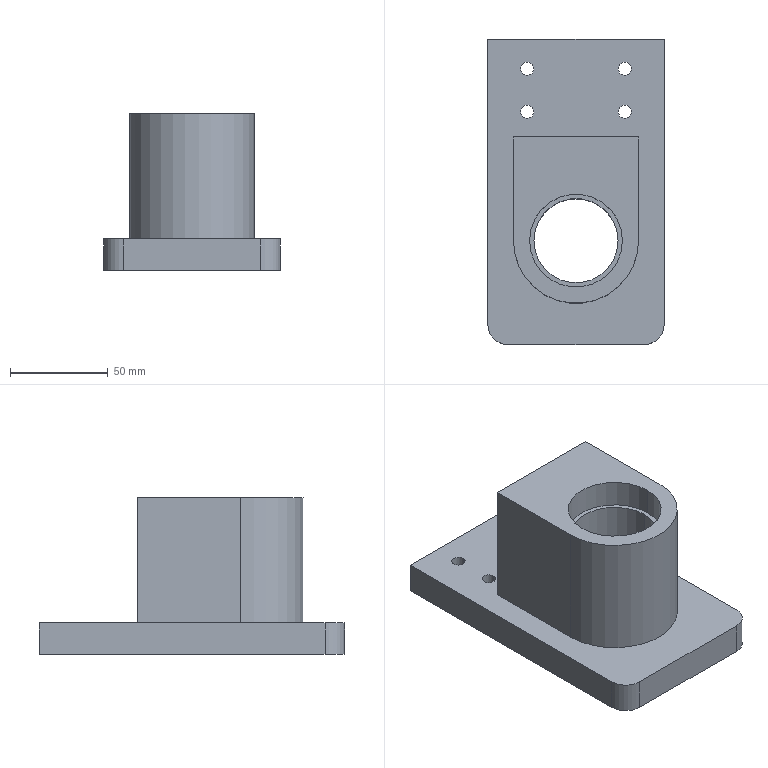NC program | NX | posted with a generic post | part box 90 x 156 x 80 mm
Lines 1 to 810 of 2108:
N10 G17 G21 G94 G90
(ADAPTIVE_MILLING , TOOL : D12-36-D12-120-3T-FINISH)
N12 T05 M6
N14 G54
N16 G17 G0 G90 X78.744 Y-62.046 S3000 M3
N18 G43 Z30. H5
N20 Z3.2
N22 G94 G1 X78.746 Y-61.896 Z2.263 F2000.
N24 X78.749 Y-61.746 Z1.892
N26 X78.751 Y-61.596 Z1.62
N28 X78.753 Y-61.446 Z1.4
N30 X78.756 Y-61.296 Z1.216
N32 X78.758 Y-61.146 Z1.058
N34 X78.76 Y-60.996 Z0.92
N36 X78.763 Y-60.846 Z0.8
N38 X78.765 Y-60.696 Z0.695
N40 X78.767 Y-60.546 Z0.602
N42 X78.77 Y-60.396 Z0.521
N44 X78.772 Y-60.246 Z0.45
N46 X78.774 Y-60.096 Z0.39
N48 X78.777 Y-59.946 Z0.338
N50 X78.779 Y-59.796 Z0.295
N52 X78.782 Y-59.646 Z0.261
N54 X78.784 Y-59.496 Z0.234
N56 X78.786 Y-59.346 Z0.215
N58 X78.789 Y-59.197 Z0.204
N60 X78.791 Y-59.047 Z0.2
N62 X78.82 Y-57.201
N64 G3 X77.983 Y-56.029 R1.212
N66 X74.762 Y-55.55 R13.285
N68 X65.236 Y-55.402 R193.444
N70 G1 X60.785 Y-55.4
N72 X-78.76 Y-55.399
N74 G2 X-83.906 Y-52.932 R6.712
N76 X-86.208 Y-48.01 R11.134
N78 X-86.816 Y-42.064 R32.789
N80 X-86.9 Y-29.285 R524.641
N82 G1 X-86.898 Y47.291
N84 G2 X-84.476 Y52.367 R6.698
N86 X-79.698 Y54.664 R10.957
N88 X-73.892 Y55.305 R30.703
N90 X-60.843 Y55.4 R460.922
N92 G1 X78.741 Y55.399
N94 G2 X83.892 Y52.944 R6.704
N96 X86.203 Y48.02 R11.142
N98 X86.818 Y41.985 R32.906
N100 X86.9 Y29.386 R528.978
N102 G1 X86.899 Y-47.241
N104 G2 X84.478 Y-52.363 R6.699
N106 X79.822 Y-54.481 R9.521
N108 X74.441 Y-54.838 R30.69
N110 G1 X63.303 Y-54.802
N112 X-76.33 Y-54.8
N114 G2 X-83.402 Y-51.047 R8.604
N116 X-85.614 Y-45.563 R13.915
N118 X-86.224 Y-38.713 R42.06
N120 X-86.299 Y-25.843 R645.049
N122 G1 X-86.298 Y44.918
N124 G2 X-82.556 Y51.894 R8.601
N126 X-77.072 Y54.112 R13.896
N128 X-70.357 Y54.72 R41.378
N130 X-57.488 Y54.799 R603.139
N132 G1 X76.413 Y54.798
N134 G2 X83.395 Y51.052 R8.603
N136 X85.602 Y45.614 R13.877
N138 X86.221 Y38.81 R41.342
N140 X86.299 Y26.166 R605.307
N142 G1 X86.298 Y-44.913
N144 G2 X82.262 Y-51.953 R8.28
N146 X76.935 Y-53.785 R13.806
N148 X70.203 Y-54.183 R49.593
N150 G1 X60.966 Y-54.2
N152 X-74.139 Y-54.199
N154 G2 X-83.054 Y-49.203 R9.955
N156 X-85.085 Y-43.278 R16.664
N158 X-85.637 Y-35.79 R53.798
N160 X-85.699 Y-22.92 R771.076
N162 G1 X-85.697 Y42.759
N164 G2 X-80.83 Y51.476 R9.919
N166 X-75.008 Y53.546 R16.303
N168 X-67.793 Y54.125 R49.758
N170 X-55.733 Y54.198 R669.374
N172 G1 X74.254 Y54.197
N174 G2 X83.001 Y49.286 R9.929
N176 X85.082 Y43.287 R16.583
N178 X85.634 Y35.889 R53.121
N180 X85.699 Y23.514 R746.255
N182 G1 X85.697 Y-42.753
N184 G2 X80.99 Y-51.128 R9.462
N186 X75.313 Y-53.072 R15.567
N188 X68.315 Y-53.556 R50.706
N190 X57.426 Y-53.6 R730.196
N192 G1 X-72.143 Y-53.599
N194 G2 X-77.204 Y-52.712 R12.671
N196 X-82.743 Y-47.364 R11.177
N198 X-84.575 Y-41.035 R19.763
N200 X-85.055 Y-32.729 R71.078
N202 X-85.098 Y-20.849 R784.904
N204 G1 X-85.097 Y40.643
N206 G2 X-84.246 Y45.621 R12.736
N208 X-78.978 Y51.184 R11.121
N210 X-72.756 Y53.043 R19.317
N212 X-64.722 Y53.547 R65.924
N214 X-52.348 Y53.598 R780.815
N216 G1 X72.228 Y53.597
N218 G2 X77.448 Y52.603 R12.37
N220 X82.845 Y47.158 R11.284
N222 X84.58 Y40.988 R20.098
N224 X85.056 Y32.636 R72.038
N226 X85.098 Y20.756 R788.507
N228 G1 X85.097 Y-40.729
N230 G2 X84.056 Y-45.889 R11.634
N232 X78.8 Y-50.936 R10.918
N234 X72.785 Y-52.561 R19.541
N236 X64.565 Y-52.971 R75.162
N238 G1 X54.665 Y-52.999
N240 X-70.27 Y-52.998
N242 G2 X-75.034 Y-52.432 R16.302
N244 X-81.817 Y-46.775 R11.527
N246 X-83.833 Y-40.507 R19.359
N248 X-84.421 Y-32.661 R58.973
N250 X-84.498 Y-18.666 R784.874
N252 G1 X-84.497 Y38.799
N254 G2 X-83.896 Y43.647 R16.065
N256 X-78.296 Y50.305 R11.54
N258 X-71.984 Y52.336 R19.354
N260 X-63.687 Y52.932 R61.525
N262 X-50.322 Y52.998 R781.592
N264 G1 X70.248 Y52.997
N266 G2 X75.055 Y52.424 R16.332
N268 X81.805 Y46.792 R11.526
N270 X83.844 Y40.427 R19.457
N272 X84.422 Y32.624 R59.718
N274 X84.498 Y18.629 R783.097
N276 G1 Y-38.568
N278 G2 X84.002 Y-43.116 R16.267
N280 X78.502 Y-49.825 R11.138
N282 X72.349 Y-51.79 R18.685
N284 X64.409 Y-52.341 R59.727
N286 X51.539 Y-52.399 R783.347
N288 G1 X-68.588 Y-52.398
N290 G2 X-73.458 Y-51.926 R19.844
N292 X-81.067 Y-45.937 R12.014
N294 X-83.192 Y-39.415 R19.987
N296 X-83.81 Y-31.48 R59.317
N298 X-83.897 Y-17.126 R701.79
N300 G1 Y36.818
N302 G2 X-83.519 Y41.563 R22.012
N304 X-77.523 Y49.518 R11.986
N306 X-70.974 Y51.682 R19.82
N308 X-62.906 Y52.312 R59.386
N310 X-48.416 Y52.397 R728.416
N312 G1 X68.628 Y52.396
N314 G2 X73.54 Y51.904 R19.499
N316 X81.061 Y45.944 R12.015
N318 X83.19 Y39.418 R20.005
N320 X83.811 Y31.439 R59.522
N322 X83.898 Y17.084 R709.817
N324 G1 X83.897 Y-36.903
N326 G2 X83.464 Y-41.596 R19.529
N328 X77.634 Y-49.061 R11.67
N330 X71.154 Y-51.15 R19.498
N332 X63.081 Y-51.73 R61.116
N334 X49.716 Y-51.799 R780.767
N336 G1 X-66.698 Y-51.798
N338 G2 X-71.718 Y-51.45 R26.207
N340 X-80.382 Y-45.044 R12.479
N342 X-82.546 Y-38.442 R20.584
N344 X-83.208 Y-30.06 R60.908
N346 X-83.297 Y-15.57 R715.335
N348 G1 Y35.288
N350 G2 X-82.922 Y40.35 R25.207
N352 X-76.551 Y48.878 R12.477
N354 X-70.001 Y51.036 R20.509
N356 X-61.934 Y51.698 R58.838
N358 X-46.95 Y51.797 R655.338
N360 G1 X66.783 Y51.796
N362 G2 X71.845 Y51.422 R25.242
N364 X80.386 Y45.034 R12.482
N366 X82.554 Y38.388 R20.672
N368 X83.214 Y29.826 R62.385
N370 X83.297 Y14.976 R792.259
N372 G1 X83.296 Y-35.418
N374 G2 X82.894 Y-40.252 R22.501
N376 X76.659 Y-48.398 R12.187
N378 X70.029 Y-50.517 R20.369
N380 X61.733 Y-51.124 R62.801
N382 X47.873 Y-51.198 R786.816
N384 G1 X-65.393 Y-51.197
N386 G2 X-70.594 Y-50.846 R28.57
N388 X-79.773 Y-44.062 R12.936
N390 X-81.966 Y-37.141 R21.65
N392 X-82.606 Y-28.757 R64.582
N394 X-82.697 Y-13.412 R754.195
N396 G1 X-82.696 Y33.533
N398 G2 X-82.414 Y38.695 R32.746
N400 X-75.568 Y48.269 R12.946
N402 X-68.958 Y50.414 R21.294
N404 X-60.308 Y51.104 R62.262
N406 X-46.314 Y51.196 R680.311
N408 G1 X65.433 Y51.195
N410 G2 X70.677 Y50.828 R27.974
N412 X79.767 Y44.068 R12.929
N414 X81.957 Y37.193 R21.608
N416 X82.603 Y28.854 R63.797
N418 X82.697 Y13.375 R734.281
N420 G1 X82.696 Y-33.528
N422 G2 X82.382 Y-38.642 R29.36
N424 X75.682 Y-47.766 R12.669
N426 X68.974 Y-49.887 R21.182
N428 X60.858 Y-50.508 R62.429
N430 X46.369 Y-50.598 R707.695
N432 G1 X-63.548 Y-50.597
N434 G2 X-69.026 Y-50.324 R37.448
N436 X-79.16 Y-43.126 R13.367
N438 X-81.344 Y-36.157 R22.372
N440 X-82.009 Y-27.278 R67.438
N442 X-82.096 Y-11.934 R807.751
N444 G1 Y32.273
N446 G2 X-81.787 Y37.749 R34.473
N448 X-74.694 Y47.622 R13.334
N450 X-67.864 Y49.809 R22.043
N452 X-59.168 Y50.499 R64.313
N454 X-43.689 Y50.596 R721.536
N456 G1 X63.588
N458 G2 X69.066 Y50.316 R36.796
N460 X79.153 Y43.134 R13.361
N462 X81.341 Y36.165 R22.362
N464 X82.011 Y27.196 R67.926
N466 X82.096 Y11.852 R816.076
N468 G1 X82.095 Y-32.268
N470 G2 X81.757 Y-37.651 R31.076
N472 X74.879 Y-47.065 R13.06
N474 X68.177 Y-49.225 R21.524
N476 X59.706 Y-49.902 R62.329
N478 X44.226 Y-49.997 R714.416
N480 G1 X-62.288
N482 G2 X-67.991 Y-49.717 R40.149
N484 X-78.555 Y-42.201 R13.741
N486 X-80.713 Y-35.264 R22.964
N488 X-81.39 Y-26.747 R65.571
N490 X-81.496 Y-11.762 R651.059
N492 G1 X-81.495 Y30.923
N494 G2 X-81.189 Y36.669 R38.015
N496 X-73.773 Y47.017 R13.714
N498 X-66.667 Y49.229 R22.976
N500 X-57.969 Y49.897 R67.552
N502 X-42.129 Y49.996 R736.146
N504 G1 X62.328 Y49.995
N506 G2 X68.031 Y49.71 R39.561
N508 X78.549 Y42.208 R13.732
N510 X80.711 Y35.271 R22.949
N512 X81.394 Y26.575 R66.277
N514 X81.496 Y10.735 R711.576
N516 G1 X81.495 Y-30.603
N518 G2 X81.221 Y-36.171 R38.784
N520 X73.889 Y-46.485 R13.489
N522 X66.821 Y-48.664 R22.713
N524 X57.896 Y-49.314 R69.395
N526 X43.002 Y-49.397 R809.845
N528 G1 X-60.983 Y-49.396
N530 G2 X-66.868 Y-49.129 R44.602
N532 X-74.889 Y-45.447 R14.199
N534 X-79.033 Y-38.723 R16.315
N536 X-80.49 Y-31.139 R32.791
N538 X-80.872 Y-20.124 R139.977
N540 G1 X-80.896 Y-9.234
N542 X-80.894 Y29.753
N544 G2 X-80.582 Y35.679 R40.195
N546 X-72.879 Y46.412 R14.054
N548 X-65.761 Y48.607 R23.562
N550 X-56.794 Y49.296 R68.958
N552 X-40.955 Y49.395 R748.954
N554 G1 X61.023
N556 G2 X66.863 Y49.128 R44.446
N558 X74.88 Y45.453 R14.209
N560 X79.047 Y38.676 R16.34
N562 X80.497 Y31.046 R33.066
N564 X80.873 Y20.076 R141.953
N566 G1 X80.896 Y9.186
N568 X80.895 Y-29.343
N570 G2 X80.623 Y-35.092 R42.138
N572 X73.026 Y-45.853 R13.845
N574 X65.819 Y-48.053 R23.381
N576 X56.714 Y-48.711 R71.35
N578 X41.37 Y-48.797 R818.597
N580 G1 X-59.895 Y-48.795
N582 G2 X-65.914 Y-48.521 R46.379
N584 X-73.671 Y-45.204 R14.683
N586 X-78.237 Y-38.355 R16.127
N588 X-79.839 Y-30.619 R31.59
N590 X-80.26 Y-20.326 R122.891
N592 G1 X-80.295 Y-7.951
N594 X-80.294 Y28.493
N596 G2 X-80. Y34.556 R44.605
N598 X-76.373 Y42.544 R14.544
N600 X-69.48 Y46.87 R16.497
N602 X-61.813 Y48.368 R32.94
N604 X-50.753 Y48.769 R137.226
N606 G1 X-39.368 Y48.795
N608 X59.872 Y48.794
N610 G2 X65.847 Y48.528 R47.338
N612 X73.454 Y45.384 R14.773
N614 X78.155 Y38.573 R15.921
N616 X79.806 Y30.941 R30.619
N618 X80.26 Y20.334 R118.142
N620 G1 X80.295 Y7.959
N622 X80.294 Y-28.191
N624 G2 X80.021 Y-34.075 R44.837
N626 X76.589 Y-41.862 R14.383
N628 X69.931 Y-46.197 R16.037
N630 X62.277 Y-47.759 R31.484
N632 X52.073 Y-48.164 R123.977
N634 G1 X40.193 Y-48.196
N636 X-58.643 Y-48.195
N638 G2 X-64.888 Y-47.926 R50.672
N640 X-72.348 Y-45.015 R15.269
N642 X-77.359 Y-38.19 R15.842
N644 X-79.125 Y-30.672 R29.303
N646 X-79.641 Y-20.7 R101.502
N648 X-79.695 Y-6.84 R852.131
N650 G1 X-79.693 Y27.233
N652 G2 X-79.413 Y33.477 R49.262
N654 X-76.343 Y41.067 R15.153
N656 X-69.612 Y45.89 R15.949
N658 X-62.046 Y47.639 R29.663
N660 X-51.623 Y48.148 R106.967
N662 X-38.258 Y48.195 R853.459
N664 G1 X58.638 Y48.193
N666 G2 X64.839 Y47.931 R51.301
N668 X72.203 Y45.121 R15.335
N670 X77.286 Y38.365 R15.712
N672 X79.09 Y30.951 R28.611
N674 X79.64 Y20.711 R98.418
N676 X79.695 Y6.851 R848.383
N678 G1 X79.694 Y-26.958
N680 G2 X79.428 Y-33.023 R48.902
N682 X76.439 Y-40.501 R14.961
N684 X69.737 Y-45.326 R15.741
N686 X62.35 Y-47.041 R29.164
N688 X52.422 Y-47.545 R101.633
N690 X38.562 Y-47.596 R861.807
N692 G1 X-57.383 Y-47.595
N694 G2 X-63.899 Y-47.33 R55.188
N696 X-71.153 Y-44.697 R15.837
N698 X-76.579 Y-37.764 R15.772
N700 X-78.459 Y-30.232 R28.522
N702 X-79.032 Y-20.128 R95.293
N704 X-79.094 Y-5.279 R868.575
N706 G1 X-79.093 Y25.973
N708 G2 X-78.823 Y32.444 R53.936
N710 X-76.123 Y39.756 R15.774
N712 X-69.172 Y45.118 R15.833
N714 X-61.457 Y46.993 R29.079
N716 X-51.081 Y47.54 R101.682
N718 X-37.221 Y47.594 R853.414
N720 G1 X57.378 Y47.593
N722 G2 X63.938 Y47.323 R54.641
N724 X71.298 Y44.592 R15.755
N726 X76.614 Y37.676 R15.849
N728 X78.465 Y30.181 R28.782
N730 X79.031 Y20.166 R95.406
N732 X79.094 Y5.317 R866.271
N734 G1 X79.093 Y-25.698
N736 G2 X78.829 Y-32.034 R52.824
N738 X76.048 Y-39.412 R15.491
N740 X69.233 Y-44.574 R15.744
N742 X61.729 Y-46.396 R28.737
N744 X51.849 Y-46.936 R96.853
N746 X37.494 Y-46.995 R854.102
N748 G1 X-56.123 Y-46.994
N750 G2 X-62.82 Y-46.746 R61.276
N752 X-69.968 Y-44.353 R16.518
N754 X-75.793 Y-37.351 R15.729
N756 X-77.791 Y-29.804 R27.783
N758 X-78.413 Y-20.064 R86.879
N760 X-78.494 Y-4.224 R858.423
N762 G1 X-78.493 Y24.591
N764 G2 X-78.238 Y31.377 R60.879
N766 X-75.835 Y38.495 R16.467
N768 X-68.951 Y44.248 R15.694
N770 X-61.458 Y46.27 R27.42
N772 X-51.585 Y46.912 R85.521
N774 X-35.746 Y46.994 R856.81
N776 G1 X56.163 Y46.993
N778 G2 X62.815 Y46.745 R61.002
N780 X70.044 Y44.302 R16.495
N782 X75.806 Y37.316 R15.755
N784 X77.808 Y29.676 R28.012
N786 X78.413 Y20.025 R88.14
N788 X78.494 Y4.186 R859.617
N790 G1 X78.493 Y-24.438
N792 G2 X78.25 Y-30.91 R59.153
N794 X75.806 Y-38.086 R16.239
N796 X68.83 Y-43.781 R15.648
N798 X61.268 Y-45.732 R27.995
N800 X51.255 Y-46.327 R91.402
N802 X36.406 Y-46.395 R852.98
N804 G1 X-54.908 Y-46.394
N806 G2 X-61.786 Y-46.159 R67.27
N808 X-68.826 Y-43.967 R17.217
N810 X-75.031 Y-36.885 R15.733
N812 X-77.131 Y-29.317 R27.267
N814 X-77.802 Y-19.49 R82.987
N816 X-77.893 Y-3.111 R855.513
N818 G1 Y23.363
N820 G2 X-77.652 Y30.331 R67.131
N822 X-75.377 Y37.475 R17.096
N824 X-68.474 Y43.49 R15.726
N826 X-60.823 Y45.63 R27.14
N828 X-50.997 Y46.302 R82.908
N830 X-34.618 Y46.393 R854.794
N832 G1 X54.948 Y46.392
N834 G2 X61.826 Y46.152 R66.256
N836 X68.973 Y43.876 R17.104
N838 X75.063 Y36.811 R15.784
N840 X77.166 Y29.058 R27.713
N842 X77.803 Y19.454 R85.095
N844 X77.894 Y3.075 R856.473
N846 G1 X77.893 Y-23.223
N848 G2 X77.635 Y-30.1 R61.983
N850 X75.231 Y-37.246 R16.584
N852 X68.208 Y-43.086 R15.771
N854 X60.528 Y-45.105 R28.024
N856 X50.652 Y-45.718 R89.32
N858 X35.307 Y-45.794 R850.207
N860 G1 X-54.188 Y-45.793
N862 G2 X-61.199 Y-45.522 R62.931
N864 X-68.367 Y-43.17 R17.201
N866 X-74.46 Y-36.014 R16.026
N868 X-76.528 Y-28.441 R27.895
N870 X-77.204 Y-18.39 R85.409
N872 X-77.293 Y-2.056 R859.702
N874 G1 X-77.292 Y22.643
N876 G2 X-77.036 Y29.565 R65.163
N878 X-74.786 Y36.677 R17.411
N880 X-67.734 Y42.858 R15.905
N882 X-60.004 Y45.018 R27.476
N884 X-50.403 Y45.692 R82.102
N886 X-33.573 Y45.793 R850.979
N888 G1 X53.733 Y45.792
N890 G2 X60.881 Y45.556 R71.449
N892 X67.899 Y43.446 R17.708
N894 X74.264 Y36.428 R15.784
N896 X76.493 Y28.67 R27.016
N898 X77.194 Y18.802 R81.334
N900 X77.293 Y1.972 R855.594
N902 G1 X77.292 Y-21.963
N904 G2 X77.048 Y-29.066 R68.379
N906 X74.887 Y-36.038 R17.306
N908 X67.84 Y-42.281 R15.722
N910 X60.287 Y-44.41 R27.048
N912 X50.642 Y-45.095 R80.428
N914 X33.768 Y-45.194 R855.1
N916 G1 X-53.097 Y-45.193
N918 G2 X-60.11 Y-44.945 R68.974
N920 X-67.21 Y-42.797 R17.952
N922 X-73.624 Y-35.723 R15.951
N924 X-75.861 Y-28.009 R27.1
N926 X-76.586 Y-18.142 R80.026
N928 X-76.693 Y-0.817 R834.785
N930 G1 X-76.691 Y21.563
N932 G2 X-76.447 Y28.575 R69.887
N934 X-74.315 Y35.678 R18.013
N936 X-67.121 Y42.173 R15.983
N938 X-59.399 Y44.378 R27.412
N940 X-49.711 Y45.084 R80.293
N942 X-32.387 Y45.192 R818.475
N944 G1 X53.038 Y45.191
N946 G2 X60.275 Y44.925 R67.498
N948 X67.355 Y42.711 R17.735
N950 X73.729 Y35.497 R16.055
N952 X75.884 Y27.853 R27.648
N954 X76.585 Y18.164 R80.897
N956 X76.693 Y0.84 R827.116
N958 G1 X76.691 Y-21.27
N960 G2 X76.43 Y-28.327 R65.795
N962 X74.174 Y-35.445 R17.463
N964 X67.035 Y-41.681 R15.962
N966 X59.43 Y-43.805 R27.532
N968 X49.515 Y-44.497 R82.744
N970 X32.64 Y-44.594 R862.85
N972 G1 X-51.93 Y-44.592
N974 G2 X-59.302 Y-44.337 R72.452
N976 X-66.375 Y-42.235 R18.326
N978 X-73.011 Y-34.969 R16.111
N980 X-75.231 Y-27.347 R27.285
N982 X-75.977 Y-17.527 R78.617
N984 X-76.092 Y0.293 R793.306
N986 G1 X-76.091 Y20.423
N988 G2 X-75.841 Y27.75 R73.341
N990 X-73.737 Y34.869 R18.385
N992 X-66.424 Y41.533 R16.115
N994 X-58.794 Y43.739 R27.435
N996 X-49.108 Y44.474 R78.604
N998 X-31.244 Y44.592 R783.615
N1000 G1 X51.976 Y44.591
N1002 G2 X59.258 Y44.34 R72.647
N1004 X66.373 Y42.234 R18.37
N1006 X72.988 Y35.011 R16.094
N1008 X75.236 Y27.305 R27.288
N1010 X75.977 Y17.484 R79.005
N1012 X76.092 Y-0.335 R799.339
N1014 G1 X76.091 Y-20.15
N1016 G2 X75.841 Y-27.342 R71.017
N1018 X73.683 Y-34.486 R18.044
N1020 X66.558 Y-40.933 R16.004
N1022 X58.978 Y-43.141 R27.083
N1024 X49.292 Y-43.878 R77.745
N1026 X31.473 Y-43.993 R787.499
N1028 G1 X-50.892 Y-43.992
N1030 G2 X-58.399 Y-43.742 R76.419
N1032 X-65.49 Y-41.703 R18.808
N1034 X-72.336 Y-34.353 R16.198
N1036 X-74.635 Y-26.471 R27.567
N1038 X-75.371 Y-16.784 R79.356
N1040 X-75.492 Y1.035 R763.152
N1042 G1 X-75.491 Y19.365
N1044 G2 X-75.248 Y26.828 R77.8
N1046 X-73.257 Y33.888 R18.95
N1048 X-65.844 Y40.84 R16.188
N1050 X-58.003 Y43.13 R27.526
N1052 X-48.317 Y43.87 R78.97
N1054 X-30.498 Y43.992 R760.908
N1056 G1 X50.832 Y43.99
N1058 G2 X58.161 Y43.764 R80.674
N1060 X65.16 Y41.874 R19.288
N1062 X72.271 Y34.481 R16.112
N1064 X74.599 Y26.695 R27.132
N1066 X75.369 Y16.832 R77.558
N1068 X75.492 Y-1.482 R777.307
N1070 G1 X75.491 Y-19.092
N1072 G2 X75.246 Y-26.42 R75.217
N1074 X73.2 Y-33.509 R18.617
N1076 X65.908 Y-40.271 R16.101
N1078 X58.068 Y-42.549 R27.409
N1080 X48.022 Y-43.286 R81.411
N1082 X30.698 Y-43.393 R839.858
N1084 G1 X-49.777 Y-43.392
N1086 G2 X-57.465 Y-43.15 R82.146
N1088 X-64.503 Y-41.225 R19.425
N1090 X-71.648 Y-33.771 R16.273
N1092 X-73.993 Y-25.909 R27.408
N1094 X-74.765 Y-16.046 R78.185
N1096 X-74.891 Y2.268 R761.574
N1098 G1 X-74.89 Y18.258
N1100 G2 X-74.655 Y25.902 R83.374
N1102 X-72.755 Y32.943 R19.539
N1104 X-65.371 Y40.098 R16.229
N1106 X-57.739 Y42.439 R26.857
N1108 X-48.24 Y43.244 R72.941
N1110 X-32.761 Y43.39 R555.777
N1112 G1 X48.884 Y43.391
N1114 G2 X56.979 Y43.194 R102.442
N1116 X63.94 Y41.498 R20.456
N1118 X71.562 Y33.939 R16.156
N1120 X73.955 Y26.138 R26.919
N1122 X74.753 Y16.458 R74.755
N1124 X74.892 Y-2.351 R713.637
N1126 G1 X74.89 Y-17.936
N1128 G2 X74.662 Y-25.4 R82.472
N1130 X72.759 Y-32.447 R19.368
N1132 X65.329 Y-39.578 R16.165
N1134 X57.501 Y-41.906 R27.27
N1136 X47.863 Y-42.664 R77.15
N1138 X29.549 Y-42.792 R743.967
N1140 G1 X-48.766 Y-42.791
N1142 G2 X-56.59 Y-42.553 R86.089
N1144 X-63.679 Y-40.663 R19.89
N1146 X-70.945 Y-33.225 R16.34
N1148 X-73.332 Y-25.465 R27.085
N1150 X-74.144 Y-15.831 R73.999
N1152 X-74.291 Y2.978 R684.08
N1154 G1 X-74.29 Y17.258
N1156 G2 X-74.061 Y24.992 R87.933
N1158 X-72.203 Y32.097 R20.08
N1160 X-64.773 Y39.421 R16.317
N1162 X-56.974 Y41.83 R26.991
N1164 X-47.295 Y42.645 R74.035
N1166 X-28.486 Y42.791 R689.641
N1168 G1 X49.244 Y42.789
N1170 G2 X56.796 Y42.531 R77.759
N1172 X63.993 Y40.499 R19.435
N1174 X71. Y33.111 R16.411
N1176 X73.38 Y25.161 R27.596
N1178 X74.159 Y15.344 R78.141
N1180 X74.291 Y-2.97 R732.035
N1182 G1 X74.29 Y-16.935
N1184 G2 X74.046 Y-24.714 R83.052
N1186 X72.109 Y-31.791 R19.515
N1188 X64.673 Y-38.927 R16.295
N1190 X56.987 Y-41.255 R27.17
N1192 X47.127 Y-42.059 R75.649
N1194 X28.813 Y-42.192 R719.228
N1196 G1 X-48.242 Y-42.19
N1198 G2 X-55.885 Y-41.941 R82.477
N1200 X-62.936 Y-40.064 R20.115
N1202 X-70.284 Y-32.604 R16.447
N1204 X-72.708 Y-24.801 R27.125
N1206 X-73.543 Y-14.989 R74.161
N1208 X-73.689 Y0.85 R572.208
N1210 G1 X-73.69 Y15.22
N1212 G2 X-73.514 Y23.541 R119.382
N1214 X-72.042 Y30.375 R22.186
N1216 X-64.27 Y38.698 R16.315
N1218 X-56.44 Y41.184 R26.737
N1220 X-46.584 Y42.039 R72.898
N1222 X-30.746 Y42.189 R561.792
N1224 G1 X46.759 Y42.19
N1226 G2 X55.08 Y42.01 R117.302
N1228 X61.953 Y40.509 R22.047
N1230 X70.201 Y32.76 R16.323
N1232 X72.669 Y25.019 R26.671
N1234 X73.521 Y15.615 R70.279
N1236 X73.689 Y-0.358 R504.918
N1238 G1 X73.691 Y-14.863
N1240 G2 X73.508 Y-23.184 R114.66
N1242 X71.974 Y-30.048 R21.628
N1244 X64.328 Y-38.122 R16.233
N1246 X56.543 Y-40.593 R26.59
N1248 X47.002 Y-41.434 R71.439
N1250 X30.534 Y-41.591 R553.488
N1252 G1 X-45.756
N1254 G2 X-54.213 Y-41.415 R123.603
N1256 X-61.138 Y-39.941 R22.599
N1258 X-69.575 Y-32.079 R16.437
N1260 X-72.089 Y-24.119 R27.054
N1262 X-72.937 Y-14.263 R74.004
N1264 X-73.089 Y2.071 R576.634
N1266 G1 X-73.09 Y14.236
N1268 G2 X-72.912 Y22.737 R122.934
N1270 X-71.429 Y29.663 R22.531
N1272 X-63.549 Y38.091 R16.449
N1274 X-55.581 Y40.595 R27.153
N1276 X-45.949 Y41.431 R73.426
N1278 X-29.481 Y41.589 R559.664
N1280 G1 X45.774 Y41.59
N1282 G2 X54.276 Y41.408 R121.061
N1284 X61.239 Y39.897 R22.399
N1286 X69.57 Y32.086 R16.441
N1288 X72.056 Y24.299 R26.848
N1290 X72.913 Y14.94 R70.184
N1292 X73.089 Y-2.068 R521.55
N1294 G1 X73.09 Y-13.873
N1296 G2 X72.906 Y-22.374 R118.271
N1298 X71.396 Y-29.245 R22.066
N1300 X63.678 Y-37.475 R16.347
N1302 X55.725 Y-39.996 R26.855
N1304 X46.094 Y-40.834 R72.805
N1306 X30.255 Y-40.99 R540.959
N1308 G1 X-44.775 Y-40.991
N1310 G2 X-53.411 Y-40.813 R127.716
N1312 X-60.259 Y-39.396 R23.155
N1314 X-68.948 Y-31.404 R16.547
N1316 X-71.485 Y-23.359 R27.312
N1318 X-72.335 Y-13.458 R74.759
N1320 X-72.489 Y2.876 R574.486
N1322 G1 X-72.488 Y14.726
N1324 G2 X-72.251 Y22.64 R91.652
N1326 X-70.444 Y29.801 R21.066
N1328 X-62.711 Y37.547 R16.668
N1330 X-54.865 Y39.984 R27.538
N1332 X-45.009 Y40.834 R74.504
N1334 X-28.675 Y40.988 R569.2
N1336 G1 X44.78 Y40.989
N1338 G2 X53.461 Y40.808 R125.706
N1340 X60.473 Y39.308 R22.832
N1342 X68.942 Y31.411 R16.554
N1344 X71.436 Y23.631 R26.979
N1346 X72.318 Y13.958 R71.083
N1348 X72.489 Y-2.87 R533.936
N1350 G1 X72.488 Y-14.36
N1352 G2 X72.251 Y-22.184 R89.679
N1354 X70.461 Y-29.26 R20.878
N1356 X62.804 Y-36.948 R16.584
N1358 X55.001 Y-39.384 R27.301
N1360 X45.46 Y-40.226 R72.598
N1362 X29.486 Y-40.389 R524.293
N1364 G1 X-43.834 Y-40.391
N1366 G2 X-52.47 Y-40.223 R135.854
N1368 X-59.333 Y-38.87 R24.023
N1370 X-68.268 Y-30.834 R16.63
N1372 X-70.807 Y-23.026 R26.885
N1374 X-71.712 Y-13.266 R70.608
N1376 X-71.888 Y3.698 R526.09
N1378 X-71.831 Y18.697 R708.313
N1380 X-71.079 Y25.484 R34.037
N1382 X-62.234 Y36.82 R16.699
N1384 X-54.195 Y39.365 R27.391
N1386 X-44.205 Y40.232 R74.784
N1388 X-28.366 Y40.387 R552.509
N1390 G1 X43.874 Y40.389
N1392 G2 X52.69 Y40.205 R128.34
N1394 X59.665 Y38.739 R23.233
N1396 X68.323 Y30.725 R16.667
N1398 X70.826 Y22.908 R27.153
N1400 X71.718 Y13.101 R71.893
N1402 X71.888 Y-3.727 R538.761
N1404 X71.83 Y-18.277 R671.317
N1406 X71.064 Y-25.061 R33.382
N1408 X62.328 Y-36.218 R16.605
N1410 X54.333 Y-38.764 R27.161
N1412 X44.478 Y-39.63 R73.479
N1414 X28.64 Y-39.789 R537.326
N1416 G1 X-42.835 Y-39.79
N1418 G2 X-51.832 Y-39.611 R136.115
N1420 X-58.859 Y-38.173 R23.815
N1422 X-67.673 Y-30.108 R16.761
N1424 X-70.247 Y-22.031 R27.44
N1426 X-71.127 Y-11.998 R74.497
N1428 X-71.288 Y4.471 R562.354
N1430 X-71.219 Y18.21 R538.853
N1432 X-70.396 Y25.078 R32.749
N1434 X-61.615 Y36.169 R16.79
N1436 X-53.582 Y38.738 R27.377
N1438 X-43.728 Y39.619 R73.301
N1440 X-26.9 Y39.787 R547.732
N1442 G1 X42.865 Y39.789
N1444 G2 X51.727 Y39.617 R138.962
N1446 X58.634 Y38.256 R24.281
N1448 X67.667 Y30.115 R16.76
N1450 X70.229 Y22.123 R27.336
N1452 X71.113 Y12.406 R72.369
N1454 X71.288 Y-4.557 R532.596
N1456 X71.218 Y-17.802 R502.256
N1458 X70.408 Y-24.536 R32.392
N1460 X61.612 Y-35.615 R16.718
N1462 X53.612 Y-38.155 R27.393
N1464 X43.668 Y-39.028 R74.039
N1466 X27.829 Y-39.188 R537.79
N1468 G1 X-41.891 Y-39.19
N1470 G2 X-50.932 Y-39.018 R143.846
N1472 X-57.972 Y-37.635 R24.58
N1474 X-66.988 Y-29.559 R16.823
N1476 X-69.606 Y-21.502 R27.262
N1478 X-70.513 Y-11.561 R72.585
N1480 X-70.687 Y5.267 R534.501
N1482 X-70.615 Y17.507 R444.777
N1484 X-69.787 Y24.374 R32.983
N1486 X-60.935 Y35.553 R16.893
N1488 X-52.816 Y38.139 R27.618
N1490 X-42.782 Y39.023 R74.705
N1492 X-26.944 Y39.186 R534.083
N1494 G1 X-22.489 Y39.188
N1496 X43.406 Y39.187
N1498 G2 X51.725 Y38.954 R101.697
N1500 X58.916 Y37.245 R22.284
N1502 X67.128 Y29.285 R16.949
N1504 X69.665 Y21.153 R27.993
N1506 X70.533 Y10.983 R76.974
N1508 X70.687 Y-5.351 R582.193
N1510 X70.6 Y-17.455 R362.26
N1512 X69.672 Y-24.307 R30.354
N1514 X61.032 Y-34.944 R16.785
N1516 X52.955 Y-37.535 R27.396
N1518 X43.102 Y-38.419 R73.309
N1520 X26.274 Y-38.588 R544.919
N1522 G1 X-41.016 Y-38.589
N1524 G2 X-50.328 Y-38.405 R141.729
N1526 X-57.319 Y-37.01 R24.546
N1528 X-66.415 Y-28.802 R16.953
N1530 X-68.985 Y-20.865 R27.453
N1532 X-69.895 Y-11.24 R70.959
N1534 X-70.087 Y6.218 R509.692
N1536 X-69.985 Y17.422 R290.38
N1538 X-68.995 Y24.355 R29.855
N1540 X-60.308 Y34.911 R16.958
N1542 X-52.283 Y37.5 R27.546
N1544 X-42.702 Y38.396 R71.501
N1546 X-27.179 Y38.584 R456.05
N1548 G1 X-21.734 Y38.588
N1550 X42.451 Y38.586
N1552 G2 X50.906 Y38.357 R106.146
N1554 X58.024 Y36.724 R22.825
N1556 X66.492 Y28.648 R17.022
N1558 X69.015 Y20.689 R27.849
N1560 X69.91 Y10.837 R73.464
N1562 X70.087 Y-6.126 R532.389
N1564 X69.989 Y-16.88 R283.233
N1566 X69.016 Y-23.771 R29.851
N1568 X60.233 Y-34.391 R16.913
N1570 X52.325 Y-36.913 R27.623
N1572 X42.698 Y-37.803 R71.824
N1574 X25.735 Y-37.988 R510.592
N1576 G1 X-40.07 Y-37.989
N1578 G2 X-49.247 Y-37.826 R156.215
N1580 X-56.306 Y-36.52 R25.862
N1582 X-65.774 Y-28.179 R17.025
N1584 X-68.386 Y-20.113 R27.608
N1586 X-69.291 Y-10.533 R71.392
N1588 X-69.486 Y6.97 R504.66
N1590 X-69.35 Y17.318 R206.609
N1592 X-68.188 Y24.312 R27.498
N1594 X-59.672 Y34.276 R17.037
N1596 X-51.774 Y36.857 R27.452
N1598 X-42.062 Y37.789 R70.37
N1600 X-24.604 Y37.986 R500.31
N1602 G1 X40.031 Y37.987
N1604 G2 X49.433 Y37.811 R150.481
N1606 X56.436 Y36.471 R25.311
N1608 X65.769 Y28.183 R17.026
N1610 X68.392 Y20.071 R27.659
N1612 X69.314 Y9.906 R74.152
N1614 X69.486 Y-6.922 R544.812
N1616 X69.344 Y-16.955 R189.185
N1618 X68.167 Y-23.856 R26.859